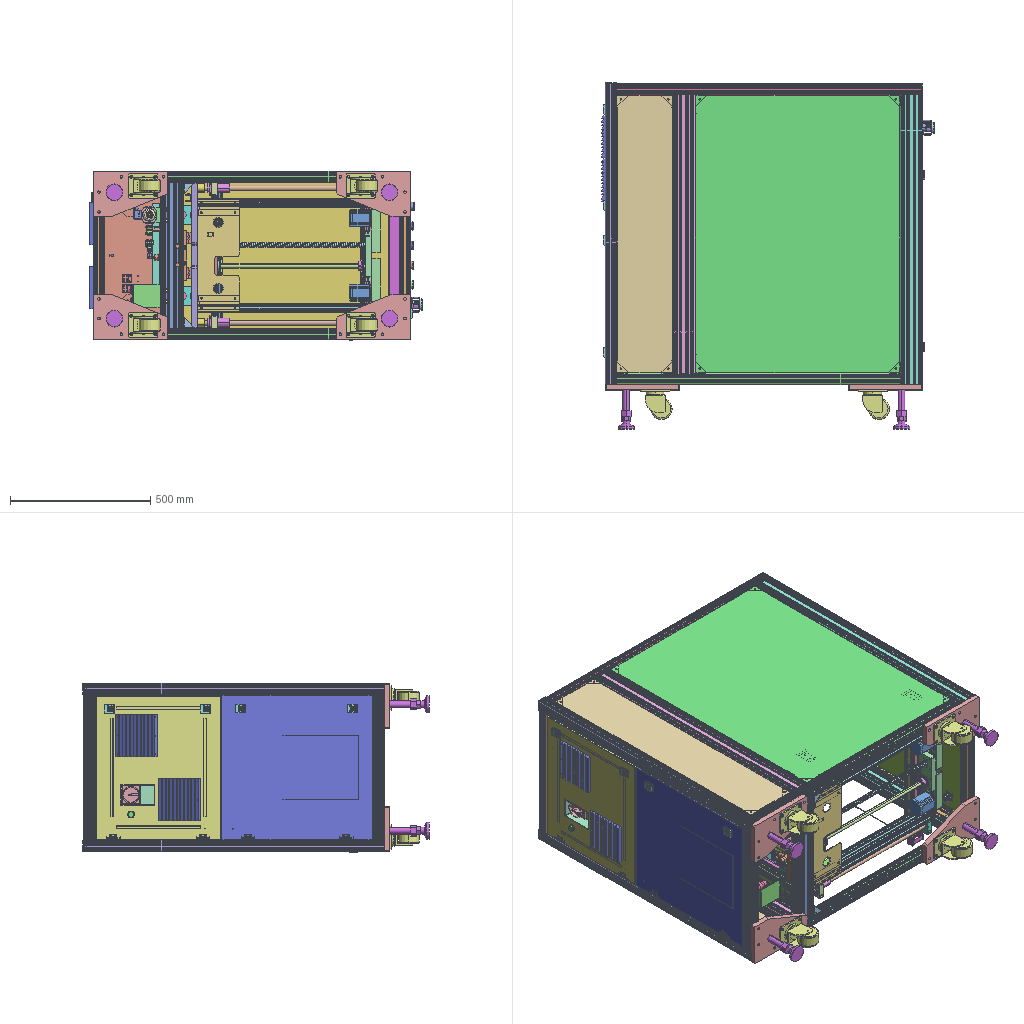Assembly | STEP file | 165 different items | 377 placed | box 1185 x 1234 x 604 mm
Parts list (item | name | quantity | parent item | size | volume):
1 | Caster support plate | x4 | - | 265 x 20 x 160 mm | 676074 mm3
2 | Fixing rod L520 | x2 | - | 520 x 40 x 80 mm | 414666 mm3
3 | Profile MK-8-4080H-L-05 4080H standard 990mm | x2 | - | 990 x 40 x 80 mm | 803657 mm3
4 | Profile MK-8-4080H-L-00 4080H standard 990mm | x2 | - | 990 x 40 x 80 mm | 803657 mm3
5 | - | x2 | - | 1030 x 40 x 80 mm | 836128 mm3
6 | Profile MK-8-4040C-L-00 4040C standard 520mm | x4 | - | 520 x 40 x 40 mm | 248689 mm3
7 | - | x2 | - | 1070 x 40 x 40 mm | 511726 mm3
8 | - | x2 | - | 1010 x 40 x 40 mm | 483031 mm3
9 | Profile MK-8-4040C-L-00 4040C standard 1086mm | x2 | - | 1086 x 40 x 40 mm | 519378 mm3
10 | - | x32 | - | 38 x 38 x 36 mm | 14409 mm3
11 | 3-inch heavy-duty caster 7223-222B | x4 | - | 112 x 105 x 88 mm | 158459 mm3
12 | - | x4 | - | 60 x 195 x 60 mm | 136685 mm3
13 | - | x2 | - | 40 x 12.4 x 40 mm | 4676 mm3
14 | - | x2 | - | 40 x 12.4 x 40 mm | 5038 mm3
15 | Door panel | x1 | - | 515 x 539 x 17 mm | 394918 mm3
16 | Hinge CL237Z3H001-01 | x6 | - | 17.5 x 48 x 18 mm | 5234 mm3
17 | - | x6 | - | 19 x 25 x 8.5 mm | 1495 mm3
18 | - | x1 | - | 230 x 270 x 19 mm | 66126 mm3
19 | - | x2 | in Lifting unit assembly | 199 x 989 x 30 mm | 288004 mm3
20 | - | x1 | in Lifting unit assembly | 199 x 519 x 30 mm | 154248 mm3
21 | Side seal plate large | x1 | in Lifting unit assembly | 988 x 728 x 30 mm | 958433 mm3
22 | - | x3 | in Lifting unit assembly | 71.855 x 71.5 x 21.7 mm | 42318 mm3
23 | Limit switch mounting plate | x2 | in Lifting unit assembly | 40 x 28 x 31 mm | 4364 mm3
24 | Cylinder fixing plate | x1 | in Lifting assembly | 95 x 15 x 180 mm | 203392 mm3
25 | Slider fixing plate | x1 | in Lifting assembly | 520 x 20 x 250 mm | 2234744 mm3
26 | Fixing block 1 | x2 | in Lifting assembly | 19 x 37 x 65 mm | 22556 mm3
27 | - | x1 | in Lifting assembly | 133 x 24 x 24 mm | 49135 mm3
28 | - | x1 | in Lifting assembly | 55 x 17 x 83 mm | 68793 mm3
29 | - | x2 | in Lifting assembly | 5.6 x 26 x 26 mm | 1190 mm3
30 | - | x2 | in Lifting assembly | 80 x 17 x 55 mm | 50244 mm3
31 | - | x2 | in Lifting assembly | 11.2 x 60 x 13 mm | 5055 mm3
32 | Fixing block 2 | x2 | in Lifting assembly | 40 x 35 x 35 mm | 25797 mm3
33 | - | x2 | in Lifting assembly | 68.92 x 68.92 x 20.5 mm | 34820 mm3
34 | - | x2 | in Lifting assembly | 12 x 42 x 42 mm | 7887 mm3
35 | - | x2 | in Support rail unit SBR30S2A+850L | 60 x 52 x 850 mm | 1179797 mm3
36 | - | x4 | in Support rail unit SBR30S2A+850L | 70 x 56 x 70 mm | 208407 mm3
37 | - | x5 | in Lifting assembly, Lifting unit assembly | 37.34 x 12.127 x 16.625 mm | 2631 mm3
38 | - | x4 | in Lifting assembly | 20 x 1 x 9 mm | 97.65 mm3
39 | - | x2 | in Lifting assembly | 16 x 16 x 8 mm | 1375 mm3
40 | - | x1 | in Lifting assembly | 494 x 75 x 75 mm | 957901 mm3
41 | Speed control valve with pilot-operated air lock ASP530F-03-08S | x1 | in Lifting assembly | 39.4 x 55.1 x 62.8 mm | 28936 mm3
42 | - | x1 | in Lifting assembly | 22.174 x 25.3 x 13.2 mm | 2514 mm3
43 | - | x1 | in Lifting assembly | 29.502 x 42.5 x 15.002 mm | 6910 mm3
44 | Speed control valve AS3201F-03-08SA | x1 | in Lifting assembly | 23 x 45.4 x 41 mm | 14301 mm3
45 | - | x2 | in Lifting assembly A_right | 620 x 30 x 60.001 mm | 358896 mm3
46 | Bottom adapter plate | x1 | in Lifting assembly A_right | 405 x 150 x 3 mm | 157925 mm3
47 | - | x2 | in Lifting assembly A_right | 60 x 12.2 x 30 mm | 5483 mm3
48 | Bearing fixing plate | x1 | - | 180 x 21 x 68 mm | 190682 mm3
49 | - | x1 | - | 170 x 21 x 57 mm | 135678 mm3
50 | - | x1 | - | 23 x 23 x 31.4 mm | 3535 mm3
51 | - | x1 | - | 16 x 647 x 16 mm | 120315 mm3
52 | - | x1 | - | 50.395 x 50.132 x 19 mm | 15455 mm3
53 | - | x1 | - | 50.395 x 50.132 x 19.5 mm | 13040 mm3
54 | - | x1 | - | 9 x 37 x 37 mm | 4601 mm3
55 | Shaft circlip type A 20 | x1 | - | 22.5 x 25.161 x 1 mm | 155.824 mm3
56 | Key 2 | x1 | - | 3.9 x 5.5 x 15 mm | 300.753 mm3
57 | - | x4 | - | 31 x 9 x 31 mm | 3611 mm3
58 | Deep groove ball bearing 606-ZZ | x8 | - | 6 x 17 x 17 mm | 776.566 mm3
59 | - | x8 | - | 18.3 x 17.603 x 1 mm | 85.781 mm3
60 | Chain sprocket spacer | x4 | - | 15 x 15 x 6.2 mm | 541.108 mm3
61 | - | x1 | - | 22 x 22 x 8 mm | 1773 mm3
62 | Bearing baffle | x2 | - | 40 x 30 x 2 mm | 1364 mm3
63 | Bearing 6000Z_P5_BONA_eco | x2 | - | 26 x 26 x 8 mm | 2544 mm3
64 | Bearing support plate | x1 | - | 12 x 35 x 135 mm | 43258 mm3
65 | -02 nut SFU01604-4 | x1 | - | 40 x 40 x 48 mm | 25660 mm3
66 | -01 screw pair SFUR1604-648 | x1 | - | 16 x 16 x 648 mm | 118967 mm3
67 | - | x1 | - | 13.6 x 15.973 x 1 mm | 68.14 mm3
68 | PN_0001 bearing 6001ZZ | x2 | - | 28 x 28 x 8 mm | 3776 mm3
69 | Motor fixing plate 2 | x2 | in Lifting assembly A_right | 68 x 152 x 35 mm | 46618 mm3
70 | - | x2 | in Lifting assembly A_right | 122.93 x 36.98 x 8 mm | 5373 mm3
71 | Stepper motor 24HS8404-10PJ3 | x2 | in Lifting assembly A_right | 60 x 96 x 60 mm | 237550 mm3
72 | Sliding plate 2 | x2 | in Lifting assembly A_right | 70 x 19 x 50 mm | 40709 mm3
73 | - | x2 | in Lifting assembly A_right | 80 x 54 x 38 mm | 45928 mm3
74 | Guide rod fixing plate 2 | x2 | in Lifting assembly A_right | 65 x 19 x 45 mm | 44231 mm3
75 | Guide shaft 2 | x2 | in Lifting assembly A_right | 20 x 20 x 616 mm | 193311 mm3
76 | - | x1 | in Lifting assembly A_right | 150 x 175 x 30 mm | 90977 mm3
77 | Right-angle fixing plate A | x1 | in Lifting assembly A_right | 150 x 175 x 30 mm | 91369 mm3
78 | - | x2 | in Lifting assembly A_right | 17.5 x 18 x 17.5 mm | 1873 mm3
79 | - | x2 | in Lifting assembly A_right | 37 x 19 x 37 mm | 15386 mm3
80 | - | x2 | in Lifting assembly A_right | 30 x 25 x 30 mm | 10205 mm3
81 | - | x1 | in Lifting assembly A_right | 22.7 x 14.9 x 13.4 mm | 1660 mm3
82 | - | x1 | in Lifting assembly A_right | 19.5 x 18 x 15 mm | 668.205 mm3
83 | - | x1 | in Lifting assembly A_right | 99 x 14.979 x 14.996 mm | 5984 mm3
84 | I/O distribution box 23N4S1 | x1 | in Lifting assembly A_right | 27.753 x 76.75 x 11.974 mm | 1445 mm3
85 | - | x4 | in Lifting assembly A_right | - | -
86 | - | x2 | in Lifting assembly A_right | 3 x 3 x 14 mm | 119.894 mm3
87 | Conveyor front chain guide groove L590 | x1 | in Conveyor assembly_right | 35 x 55 x 590 mm | 449690 mm3
88 | Conveyor rear chain guide groove L590 | x1 | in Conveyor assembly_right | 35 x 55 x 590 mm | 449690 mm3
89 | - | x2 | in Conveyor assembly_right | 9 x 490 x 20.4 mm | 77235 mm3
90 | - | x2 | in Conveyor assembly_right | 34.8 x 1 x 54.8 mm | 1804 mm3
91 | - | x2 | in Conveyor assembly_right | 34.8 x 1 x 54.8 mm | 1804 mm3
92 | - | x4 | - | 25 x 8.5 x 25 mm | 1521 mm3
93 | Driven guide wheel connector | x4 | in Conveyor assembly_right | 36 x 5 x 10.6 mm | 1667 mm3
94 | - | x4 | in Conveyor assembly_right | 15 x 15 x 3.5 mm | 281.21 mm3
95 | - | x2 | in Conveyor assembly_right | 18.325 x 9 x 17.4 mm | 854.513 mm3
96 | 06B side guide chain buckle | x2 | in Conveyor assembly_right | 15 x 1 x 7 mm | 49.292 mm3
97 | - | x2 | in Conveyor assembly_right, Lifting assembly A_right | 11.2 x 58.715 x 345.215 mm | 7993 mm3
98 | - | x2 | in Conveyor assembly_right | 20 x 10 x 20 mm | 2790 mm3
99 | Fixing plate 3 | x2 | in Conveyor assembly_right | 10 x 50 x 50 mm | 18064 mm3
100 | Photoelectric fixing plate 3 | x1 | in Conveyor assembly_right | 33 x 38 x 78 mm | 5566 mm3
101 | Photoelectric adapter plate 4 | x1 | in Lifting assembly A_right | 55 x 32 x 23.5 mm | 3494 mm3
102 | Adapter plate 3 | x4 | in Lifting unit assembly | 32 x 35 x 40 mm | 7142 mm3
103 | - | x2 | in Lifting unit assembly | 55 x 24.5 x 48.5 mm | 5670 mm3
104 | - | x1 | in Lifting unit assembly | 60 x 100 x 1.5 mm | 8744 mm3
105 | Polyurethane anti-collision column 2 | x4 | in Lifting unit assembly | 35 x 30 x 35 mm | 26422 mm3
106 | Cable carrier adapter plate 2 | x1 | in Lifting unit assembly | 35 x 35 x 37 mm | 4434 mm3
107 | - | x4 | in Lifting unit assembly | 30 x 30 x 1 mm | 412.566 mm3
108 | - | x4 | in Lifting unit assembly | 22 x 20 x 80 mm | 6135 mm3
109 | - | x2 | in Lifting unit assembly | 40 x 20 x 28 mm | 6776 mm3
110 | - | x1 | in Lifting unit assembly | 141.7 x 32.5 x 16 mm | 47379 mm3
111 | - | x1 | in Lifting unit assembly | 30 x 30 x 44.8 mm | 24470 mm3
112 | Pressure regulator filter GFR300-08-N | x1 | in Lifting unit assembly | - | -
113 | Hand slide valve HSV06 | x1 | in Lifting unit assembly | 27.5 x 27.5 x 50 mm | 15432 mm3
114 | Cylinder lock MS813-Shengjiu | x6 | in Lifting unit assembly | 58.793 x 35 x 31.6 mm | 16415 mm3
115 | Hydraulic buffer ACJ-1412 | x2 | in Lifting unit assembly | 19 x 100 x 21.289 mm | 13894 mm3
116 | - | x1 | - | 519 x 150 x 79 mm | 247371 mm3
117 | - | x1 | - | 40 x 40 x 48 mm | 24355 mm3
118 | - | x1 | - | 30 x 30 x 33 mm | 18043 mm3
119 | Pushbutton head LA42PD-Y | x2 | - | 30 x 30 x 76 mm | 18961 mm3
120 | Pushbutton head LA42PD-S | x1 | - | 30 x 30 x 33 mm | 18043 mm3
121 | - | x5 | - | 41 x 30 x 22 mm | 6377 mm3
122 | - | x5 | - | 32 x 10 x 42 mm | 10410 mm3
123 | Switch contact LA42-10-NO | x5 | - | 32 x 10 x 42 mm | 10410 mm3
124 | Emergency stop protective ring J-V | x1 | - | 47.915 x 30.4 x 47.915 mm | 9284 mm3
125 | Button cover plate | x1 | - | 519 x 39.5 x 206 mm | 125183 mm3
126 | Flashing buzzer AD17-SML-DC24V | x1 | - | 29 x 29 x 63 mm | 18875 mm3
127 | - | x1 | in Front sheet-metal door welded assembly | 515 x 796 x 17 mm | 556251 mm3
128 | - | x2 | in Front sheet-metal door welded assembly | 60 x 10 x 490 mm | 55944 mm3
129 | Electrical cabinet support plate | x1 | in Lifting unit assembly | 28 x 370 x 23 mm | 51078 mm3
130 | - | x2 | in Lifting unit assembly | 55 x 18 x 52 mm | 5293 mm3
131 | Limit fixing plate 2 | x1 | in Lifting unit assembly | 207 x 78 x 55 mm | 153668 mm3
132 | Connector fixing plate 2 | x1 | in Lifting unit assembly | 82 x 100 x 83 mm | 26763 mm3
133 | SMEMA connector | x2 | in Lifting unit assembly | 36 x 36 x 78.52 mm | 45655 mm3
134 | Face cover reinforcing rib 300mm | x2 | - | 300 x 21 x 6 mm | 7570 mm3
135 | - | x1 | - | 513 x 444 x 17 mm | 274646 mm3
136 | - | x2 | - | 350 x 21 x 6 mm | 8832 mm3
137 | Power knob mounting sheet metal | x1 | - | 74 x 122 x 41 mm | 24069 mm3
138 | - | x1 | - | 515 x 446 x 234 mm | 856637 mm3
139 | Class B ventilation filter mesh assembly ZL-803 (7032 glue) | x2 | - | 150 x 150 x 28 mm | 421271 mm3
140 | Control system fixing plate | x2 | - | 446 x 425 x 18 mm | 245891 mm3
141 | Power adapter plate 2 | x2 | - | 398 x 7.5 x 143 mm | 93935 mm3
142 | Power filter DL-10T1 | x1 | - | 89.5 x 36.5 x 51.5 mm | 121807 mm3
143 | Axial fan 1238A2MBL | x1 | - | 120 x 120 x 38 mm | 111801 mm3
144 | Six-position grounding copper block | x2 | - | 30.3 x 30.2 x 15 mm | 7115 mm3
145 | - | x1 | - | 24 x 37.7 x 24 mm | 7790 mm3
146 | - | x1 | - | 65.5 x 92 x 65.5 mm | 250369 mm3
147 | - | x1 | - | 54 x 38 x 11.5 mm | 8666 mm3
148 | Switching power supply LRS-50-24 (Mean Well) | x1 | - | 99 x 30 x 82 mm | 213867 mm3
149 | PLC module FX5U-32MT_ES | x1 | - | 150 x 96.4 x 84.9 mm | 980252 mm3
150 | Feed-through terminal block PT2,5-QUATTRO-3209578 | x20 | - | 5.15 x 72.2 x 35.25 mm | 9561 mm3
151 | Schneider miniature circuit breaker iDPNN-1P+N-C10A | x1 | - | 17.5 x 90.6 x 73.848 mm | 76092 mm3
152 | - | x1 | - | 35.4 x 93.9 x 74.3 mm | 159125 mm3
153 | Residual current device Vigi-iC65-ELE-2P-40A-30mA-A | x1 | - | 76.2 x 105.618 x 73.908 mm | 172404 mm3
154 | Switching power supply LRS-100-48 | x1 | - | 129 x 30 x 97 mm | 340596 mm3
155 | - | x2 | - | 119 x 77.6 x 25.5 mm | 99944 mm3
156 | - | x4 | - | 50.5 x 35.3 x 9.5 mm | 9735 mm3
157 | Rail socket EA9XN310 | x1 | - | 65.5 x 80.8 x 55 mm | 247844 mm3
158 | - | x3 | - | 80.625 x 35 x 371 mm | 72614 mm3
159 | 35 cable trunking (400) 2 | x2 | - | 80.625 x 35 x 425 mm | 83190 mm3
160 | - | x2 | - | 5.5 x 35 x 350 mm | 7332 mm3
161 | LED lighting lamp QELTS-300-220 220V 300mm | x1 | - | 37 x 33.2 x 378 mm | 378498 mm3
162 | - | x1 | in Acrylic cover plate assembly | 822 x 540 x 5 mm | 2219396 mm3
163 | Friction strip L824 | x2 | in Acrylic cover plate assembly | 7 x 11 x 824 mm | 22001 mm3
164 | Friction strip L542 | x2 | in Acrylic cover plate assembly | 7 x 11 x 542 mm | 14387 mm3
165 | Limit switch fixing plate 2 | x1 | in Lifting unit assembly | 40 x 26 x 30 mm | 4044 mm3
Placements (level | parent | child | x y z in mm | rotation matrix by rows), first 379 of 406 lines:
1 | Lifting unit assembly | subassembly 2 | 817.116 381.543 740.825 | 1 0 0 0 1 0 0 0 1
2 | subassembly 2 | Caster support plate | 950.319 429.73 717.441 | -1 0 0 0 1 0 0 0 -1
2 | subassembly 2 | Caster support plate | 950.319 429.73 1317.441 | -1 0 0 0 -1 0 0 0 1
2 | subassembly 2 | Caster support plate | -179.681 429.73 1317.441 | 1 0 0 0 1 0 0 0 1
2 | subassembly 2 | Caster support plate | -179.681 429.73 717.441 | 1 0 0 0 -1 0 0 0 -1
2 | subassembly 2 | Fixing rod L520 | 100.319 459.73 1277.441 | 0 0 1 0 1 0 -1 0 0
2 | subassembly 2 | Fixing rod L520 | 100.319 1489.73 757.441 | 0 0 1 0 -1 0 1 0 0
2 | subassembly 2 | Profile MK-8-4080H-L-05 4080H standard 990mm | 80.319 479.73 1161.941 | 0 -1 0 1 0 0 0 0 1
2 | subassembly 2 | Profile MK-8-4080H-L-05 4080H standard 990mm | 80.319 479.73 872.941 | 0 -1 0 1 0 0 0 0 1
2 | subassembly 2 | Profile MK-8-4080H-L-00 4080H standard 990mm | 100.319 479.73 737.441 | 0 0 1 1 0 0 0 1 -0
2 | subassembly 2 | Profile MK-8-4080H-L-00 4080H standard 990mm | 100.319 479.73 1297.441 | 0 0 1 1 0 0 0 1 -0
2 | subassembly 2 | subassembly 3 | 910.319 1469.73 1297.441 | 0 0 -1 -1 0 0 0 1 0
2 | subassembly 2 | subassembly 3 | 910.319 1469.73 737.441 | 0 0 -1 -1 0 0 0 1 0
2 | subassembly 2 | Profile MK-8-4040C-L-00 4040C standard 520mm | -159.681 459.73 757.441 | 0 0 -1 0 1 0 1 0 0
2 | subassembly 2 | Profile MK-8-4040C-L-00 4040C standard 520mm | 930.319 459.73 757.441 | 0 0 -1 0 1 0 1 0 0
2 | subassembly 2 | Profile MK-8-4040C-L-00 4040C standard 520mm | -159.681 1489.73 757.441 | 0 0 -1 0 1 0 1 0 0
2 | subassembly 2 | Profile MK-8-4040C-L-00 4040C standard 520mm | 930.319 1449.73 757.441 | 0 0 -1 0 1 0 1 0 0
2 | subassembly 2 | subassembly 4 | -159.681 439.73 1297.441 | 0 -1 0 1 0 0 0 0 1
2 | subassembly 2 | subassembly 5 | -139.681 459.73 1297.441 | 1 0 0 0 1 0 0 0 1
2 | subassembly 2 | subassembly 4 | -159.681 439.73 737.441 | 0 -1 0 1 0 0 0 0 1
2 | subassembly 2 | subassembly 5 | -139.681 459.73 737.441 | 1 0 0 0 1 0 0 0 1
2 | subassembly 2 | Profile MK-8-4040C-L-00 4040C standard 1086mm | -139.681 1489.73 1297.441 | 1 0 0 0 1 0 0 0 1
2 | subassembly 2 | Profile MK-8-4040C-L-00 4040C standard 1086mm | -139.681 1489.73 737.441 | 1 0 0 0 1 0 0 0 1
2 | subassembly 2 | subassembly 6 | -139.681 479.73 737.441 | 1 0 0 0 1 0 0 0 1
2 | subassembly 2 | subassembly 6 | -139.681 1469.73 737.441 | 0 1 0 -1 0 0 0 0 1
2 | subassembly 2 | subassembly 6 | 60.319 479.73 737.291 | 0 -1 0 1 0 0 0 0 1
2 | subassembly 2 | subassembly 6 | 60.319 1469.73 737.441 | -1 0 0 0 -1 0 0 0 1
2 | subassembly 2 | subassembly 6 | 140.319 479.73 737.291 | 1 0 0 0 1 0 0 0 1
2 | subassembly 2 | subassembly 6 | 140.319 1469.73 737.441 | 0 1 0 -1 0 0 0 0 1
2 | subassembly 2 | subassembly 6 | 870.319 479.73 737.441 | 0 -1 0 1 0 0 0 0 1
2 | subassembly 2 | subassembly 6 | 870.319 479.73 1297.291 | -1 0 0 0 1 0 0 0 -1
2 | subassembly 2 | subassembly 6 | 870.319 1469.73 1297.591 | 0 -1 0 -1 0 0 0 0 -1
2 | subassembly 2 | subassembly 6 | 140.319 1469.73 1297.441 | 1 0 0 0 -1 0 0 0 -1
2 | subassembly 2 | subassembly 6 | 140.319 479.73 1297.441 | 0 1 0 1 0 0 0 0 -1
2 | subassembly 2 | subassembly 6 | -139.681 1469.73 1297.441 | 1 0 0 0 -1 0 0 0 -1
2 | subassembly 2 | subassembly 6 | -139.681 479.73 1297.441 | 0 1 0 1 0 0 0 0 -1
2 | subassembly 2 | subassembly 6 | 60.319 479.73 1297.441 | -1 0 0 0 1 0 0 0 -1
2 | subassembly 2 | subassembly 6 | 60.319 1469.73 1297.441 | 0 -1 0 -1 0 0 0 0 -1
2 | subassembly 2 | subassembly 6 | 60.319 1489.73 1277.441 | -1 0 0 0 0 -1 0 -1 -0
2 | subassembly 2 | subassembly 6 | 60.319 1489.73 757.441 | 0 -1 0 0 0 -1 1 0 -0
2 | subassembly 2 | subassembly 6 | -139.681 1489.73 757.441 | 1 0 0 0 0 -1 0 1 0
2 | subassembly 2 | subassembly 6 | 60.319 459.73 1277.441 | -1 0 0 0 0 -1 0 -1 -0
2 | subassembly 2 | subassembly 6 | 60.319 459.73 757.441 | 0 -1 0 0 0 -1 1 0 0
2 | subassembly 2 | subassembly 6 | 140.319 459.73 1277.441 | 0 1 0 0 0 -1 -1 0 0
2 | subassembly 2 | 3-inch heavy-duty caster 7223-222B | 772.319 414.73 769.941 | -1 0 0 0 1 0 0 0 -1
2 | subassembly 2 | 3-inch heavy-duty caster 7223-222B | -1.681 414.73 769.941 | -1 0 0 0 1 0 0 0 -1
2 | subassembly 2 | 3-inch heavy-duty caster 7223-222B | 772.319 414.73 1264.941 | -1 0 0 0 1 0 0 0 -1
2 | subassembly 2 | 3-inch heavy-duty caster 7223-222B | -1.681 414.73 1264.941 | -1 0 0 0 1 0 0 0 -1
2 | subassembly 2 | subassembly 7 | 875.319 279.73 1242.441 | 1 0 0 0 1 0 0 0 1
2 | subassembly 2 | subassembly 7 | 875.319 279.73 792.441 | 1 0 0 0 1 0 0 0 1
2 | subassembly 2 | subassembly 7 | -104.681 279.73 792.441 | 1 0 0 0 1 0 0 0 1
2 | subassembly 2 | subassembly 7 | -104.681 279.73 1242.441 | 1 0 0.000641 0 1 0 -0.000641 0 1
2 | subassembly 2 | subassembly 6 | 80.169 1469.73 1277.441 | 0 0 -1 0 -1 0 -1 0 0
2 | subassembly 2 | subassembly 6 | 80.169 1469.73 757.441 | 0 0 -1 -1 0 0 0 1 -0
2 | subassembly 2 | subassembly 6 | -139.681 1489.73 1277.441 | 0 1 0 0 0 -1 -1 0 0
2 | subassembly 2 | subassembly 6 | 870.319 1469.73 737.441 | -1 0 0 0 -1 0 0 0 1
2 | subassembly 2 | subassembly 6 | 140.319 459.73 757.441 | 1 0 0 0 0 -1 0 1 0
2 | subassembly 2 | subassembly 6 | 910.319 1449.73 757.441 | -1 0 0 0 0 1 0 1 -0
2 | subassembly 2 | subassembly 6 | 910.319 1449.73 1277.441 | 0 -1 0 0 0 1 -1 0 -0
2 | subassembly 2 | subassembly 6 | 910.319 459.73 757.441 | 0 -1 0 0 0 -1 1 0 0
2 | subassembly 2 | subassembly 6 | 910.319 459.73 1277.441 | 0 -1 0 0 0 1 -1 0 -0
2 | subassembly 2 | subassembly 6 | -139.681 459.73 1277.441 | 0 1 0 0 0 -1 -1 0 0
2 | subassembly 2 | subassembly 6 | -139.681 459.73 757.441 | 1 0 0 0 0 -1 0 1 0
2 | subassembly 2 | subassembly 8 | 950.519 1489.73 1297.441 | 0 -1 0 -1 0 0 0 0 -1
2 | subassembly 2 | subassembly 8 | 950.519 1489.73 737.441 | 0 -1 0 1 0 0 0 0 1
2 | subassembly 2 | subassembly 9 | -159.681 1513.93 737.441 | -1 0 0 0 -1 0 0 0 1
2 | subassembly 2 | subassembly 9 | -159.681 1513.93 1297.441 | -1 0 0 0 -1 0 0 0 1
1 | Lifting unit assembly | subassembly 10 | 953.735 1175.238 2160.396 | 0 0 1 0 -1 0 1 0 -0
2 | subassembly 10 | Door panel | -402.579 43.466 -315.1 | -1 0 0 0 -1 0 0 0 1
2 | subassembly 10 | subassembly 11 | -628.948 -156.165 -270.668 | -1 0 0 0 1 0 0 0 -1
3 | subassembly 11 | Hinge CL237Z3H001-01 | 25.631 24.631 40.182 | 1 0 0 0 1 0 0 0 1
3 | subassembly 11 | subassembly 12 | 25.631 24.631 40.182 | -1 0 0 0 1 0 0 0 -1
2 | subassembly 10 | subassembly 11 | -628.948 193.835 -270.668 | -1 0 0 0 1 0 0 0 -1
3 | subassembly 11 | Hinge CL237Z3H001-01 | 25.631 24.631 40.182 | 1 0 0 0 1 0 0 0 1
3 | subassembly 11 | subassembly 12 | 25.631 24.631 40.182 | -1 0 0 0 1 0 0 0 -1
2 | subassembly 10 | subassembly 13 | -402.579 127.966 -296.1 | -1 0 0 0 -1 0 0 0 1
1 | Lifting unit assembly | subassembly 14 | 777.434 1356.272 1459.067 | -1 0 0 0 1 0 0 0 -1
1 | Lifting unit assembly | subassembly 14 | 777.434 1356.272 2057.466 | 1 0 0 0 1 0 0 0 1
1 | Lifting unit assembly | subassembly 15 | 777.434 1890.472 1758.266 | 1 0 0 0 0 1 0 -1 0
1 | Lifting unit assembly | Side seal plate large | 1322.434 1356.272 2058.266 | 0 1 0 -1 0 0 0 0 1
1 | Lifting unit assembly | subassembly 16 | 1060.134 1830.272 1511.617 | -1 0 0 0 1 0 0 0 -1
1 | Lifting unit assembly | Limit switch mounting plate | 1047.434 1837.272 1498.767 | -1 0 0 0 1 0 0 0 -1
1 | Lifting unit assembly | Lifting assembly A_right | 994.3 1296.677 1735.039 | 1 0 0 0 1 0 0 0 1
2 | Lifting assembly A_right | Lifting assembly | -1579.962 -1409.405 569.136 | 1 0 0 0 1 0 0 0 1
3 | Lifting assembly | Cylinder fixing plate | 1508.097 974.0 -545.909 | -1 0 0 0 1 0 0 0 -1
3 | Lifting assembly | Slider fixing plate | 1573.097 1124.0 -545.909 | 0 1 0 0 0 -1 -1 0 0
3 | Lifting assembly | Fixing block 1 | 1510.597 999.0 -608.409 | 0 0 1 0 1 0 -1 0 -0
3 | Lifting assembly | Fixing block 1 | 1510.597 999.0 -483.409 | 0 0 1 0 1 0 -1 0 -0
3 | Lifting assembly | subassembly 17 | 1518.097 1526.0 -545.909 | 0 -0.2484 -0.9687 0 -0.9687 0.2484 -1 0 -0
3 | Lifting assembly | subassembly 18 | 1518.097 1476.0 -545.909 | 1 0 0 0 -1 0 0 0 -1
3 | Lifting assembly | subassembly 19 | 1518.097 1526.0 -500.309 | 0 0.3457 0.9383 0 0.9383 -0.3457 -1 0 0
3 | Lifting assembly | subassembly 19 | 1518.097 1526.0 -585.909 | 0 0.8733 0.4872 0 0.4872 -0.8733 -1 0 0
3 | Lifting assembly | subassembly 20 | 1518.097 1516.0 -578.909 | 0 0 1 -1 0 0 0 -1 0
3 | Lifting assembly | subassembly 20 | 1518.097 1516.0 -512.909 | 0 0 -1 -1 0 0 0 1 -0
3 | Lifting assembly | subassembly 21 | 1551.097 1066.5 -483.409 | 0 0 1 0 1 0 -1 0 -0
3 | Lifting assembly | subassembly 21 | 1551.097 1066.5 -608.409 | 0 0 1 0 1 0 -1 0 -0
3 | Lifting assembly | Fixing block 2 | 1555.597 1059.0 -483.409 | 0 0 1 0 -1 0 1 0 0
3 | Lifting assembly | Fixing block 2 | 1555.597 1059.0 -608.409 | 0 0 1 0 -1 0 1 0 -0
3 | Lifting assembly | subassembly 22 | 1518.097 1526.0 -608.409 | 0.601 0.7992 0 0.7992 -0.601 0 0 0 -1
3 | Lifting assembly | subassembly 23 | 1518.097 1526.0 -511.909 | 0 -0.235 -0.972 0 -0.972 0.235 -1 0 -0
3 | Lifting assembly | subassembly 23 | 1518.097 1526.0 -579.909 | 0 -0.235 -0.972 0 -0.972 0.235 -1 0 -0
3 | Lifting assembly | subassembly 22 | 1518.097 1526.0 -483.409 | -0.601 0.7992 0 -0.7992 -0.601 0 0 0 1
3 | Lifting assembly | Support rail unit SBR30S2A+850L | 1540.097 1434.0 -401.409 | 0 1 0 0 0 -1 -1 0 -0
4 | Support rail unit SBR30S2A+850L | subassembly 24 | -0.0 -0.0 -0.0 | 1 0 0 0 1 0 0 0 1
4 | Support rail unit SBR30S2A+850L | subassembly 25 | 0.0 -0.0 220.0 | 1 0 0 0 1 0 0 0 1
4 | Support rail unit SBR30S2A+850L | subassembly 25 | 0.0 -0.0 385.0 | 1 0 0 0 1 0 0 0 1
3 | Lifting assembly | Support rail unit SBR30S2A+850L | 1540.097 1434.0 -690.409 | 0 1 0 0 0 -1 -1 0 -0
4 | Support rail unit SBR30S2A+850L | subassembly 24 | -0.0 -0.0 -0.0 | 1 0 0 0 1 0 0 0 1
4 | Support rail unit SBR30S2A+850L | subassembly 25 | 0.0 -0.0 220.0 | 1 0 0 0 1 0 0 0 1
4 | Support rail unit SBR30S2A+850L | subassembly 25 | 0.0 -0.0 385.0 | 1 0 0 0 1 0 0 0 1
3 | Lifting assembly | subassembly 26 | 1496.243 1009.121 -608.409 | 0 1 0 -1 0 0 0 0 1
3 | Lifting assembly | subassembly 27 | 1485.125 1026.85 -616.834 | -0.004456 0 -1 -1 0 0.004456 0 1 0
3 | Lifting assembly | subassembly 26 | 1496.243 1009.121 -483.409 | 0 1 0 -1 0 0 0 0 1
3 | Lifting assembly | subassembly 27 | 1485.125 1026.85 -491.834 | -0.004456 0 -1 -1 0 0.004456 0 1 0
3 | Lifting assembly | subassembly 28 | 1551.097 1053.5 -483.409 | 0.6856 0.728 0 0 0 1 0.728 -0.6856 -0
3 | Lifting assembly | subassembly 28 | 1551.097 1053.5 -608.409 | 0.6856 0.728 0 0 0 1 0.728 -0.6856 -0
3 | Lifting assembly | subassembly 27 | 1551.069 1096.85 -599.984 | 0.004456 0 1 -1 0 0.004456 0 -1 -0
3 | Lifting assembly | subassembly 26 | 1539.951 1079.121 -608.409 | 0 -1 0 -1 0 0 0 0 -1
3 | Lifting assembly | subassembly 27 | 1551.069 1096.85 -474.984 | 0.004456 0 1 -1 0 0.004456 0 -1 -0
3 | Lifting assembly | subassembly 26 | 1539.951 1079.121 -483.409 | 0 -1 0 -1 0 0 0 0 -1
3 | Lifting assembly | subassembly 29 | 1518.097 1410.0 -545.909 | 0 0 -1 -1 0 0 0 1 0
3 | Lifting assembly | Speed control valve with pilot-operated air lock ASP530F-03-08S | 1485.497 1005.5 -553.409 | 0 -1 0 0 0 -1 1 0 -0
3 | Lifting assembly | subassembly 30 | 1438.247 1005.5 -553.409 | 0 -1 0 0.5 0 -0.866 0.866 0 0.5
3 | Lifting assembly | subassembly 31 | 1422.647 1031.45 -508.462 | 1 0 0 0 0.5 -0.866 0 0.866 0.5
3 | Lifting assembly | Speed control valve AS3201F-03-08SA | 1485.297 1393.5 -553.409 | 0 -1 0 0.943 0 -0.3328 0.3328 0 0.943
2 | Lifting assembly A_right | subassembly 32 | 13.135 -380.405 210.728 | 1 0 0 0 0 -1 0 1 -0
2 | Lifting assembly A_right | subassembly 32 | 13.135 -380.405 -164.272 | 1 0 0 0 0 -1 0 1 -0
2 | Lifting assembly A_right | Bottom adapter plate | 88.135 -410.405 23.228 | 0 -1 0 0 0 1 -1 0 0
2 | Lifting assembly A_right | subassembly 33 | 637.135 -380.405 210.728 | 0 -1 0 1 0 0 0 0 1
2 | Lifting assembly A_right | subassembly 33 | 637.135 -380.405 -164.272 | 0 -1 0 1 0 0 0 0 1
2 | Lifting assembly A_right | subassembly 34 | 203.126 -373.279 -397.598 | 0 -1 0 0 0 1 -1 0 0
3 | subassembly 34 | Bearing fixing plate | -418.325 -418.509 -11.126 | 1 0 0 0 1 0 0 0 1
3 | subassembly 34 | subassembly 35 | -413.325 128.491 -5.626 | 1 0 0 0 1 0 0 0 1
3 | subassembly 34 | subassembly 36 | -383.325 106.991 -12.126 | 0.8521 0.5234 0 0 0 1 0.5234 -0.8521 -0
3 | subassembly 34 | subassembly 37 | -383.325 -136.509 -12.126 | 0.5234 0 -0.8521 0 -1 0 -0.8521 0 -0.5234
3 | subassembly 34 | subassembly 38 | -383.325 -399.509 -12.126 | 0.03301 0.9995 0 0 0 -1 -0.9995 0.03301 -0
3 | subassembly 34 | subassembly 39 | -383.325 109.491 -12.126 | -0.09776 -0.9952 0 0 0 -1 0.9952 -0.09776 0
3 | subassembly 34 | subassembly 40 | -383.325 130.991 -12.126 | 0 -0.1125 0.9936 -1 0 0 0 -0.9936 -0.1125
3 | subassembly 34 | Shaft circlip type A 20 | -382.696 135.991 -11.897 | -0.342 0.9397 0 0 0 1 0.9397 0.342 -0
3 | subassembly 34 | Key 2 | -387.905 108.941 -4.67 | -0.8521 -0.5234 0 0 0 1 -0.5234 0.8521 -0
3 | subassembly 34 | subassembly 41 | -313.591 -372.036 27.854 | 0.4469 0 -0.8946 0 -1 0 -0.8946 0 -0.4469
4 | subassembly 41 | subassembly 42 | -6.597 27.473 34.415 | 1 0 0 0 1 0 0 0 1
4 | subassembly 41 | Deep groove ball bearing 606-ZZ | -6.597 26.773 34.415 | 0 1 0 -1 0 0 0 0 1
4 | subassembly 41 | subassembly 43 | -6.597 30.473 34.415 | 1 0 0 0 0 -1 0 1 -0
3 | subassembly 34 | Chain sprocket spacer | -347.325 -408.009 18.374 | -0.09332 0.9956 0 0 0 1 0.9956 0.09332 -0
3 | subassembly 34 | Chain sprocket spacer | -419.325 -408.009 18.374 | -0.09332 0.9956 0 0 0 1 0.9956 0.09332 -0
3 | subassembly 34 | subassembly 41 | -385.591 -372.036 27.854 | 0.4469 0 -0.8946 0 -1 0 -0.8946 0 -0.4469
4 | subassembly 41 | subassembly 42 | -6.597 27.473 34.415 | 1 0 0 0 1 0 0 0 1
4 | subassembly 41 | Deep groove ball bearing 606-ZZ | -6.597 26.773 34.415 | 0 1 0 -1 0 0 0 0 1
4 | subassembly 41 | subassembly 43 | -6.597 30.473 34.415 | 1 0 0 0 0 -1 0 1 -0
3 | subassembly 34 | Chain sprocket spacer | -419.325 117.991 18.374 | -0.354 -0.9352 0 0 0 -1 0.9352 -0.354 0
3 | subassembly 34 | Chain sprocket spacer | -347.325 117.991 18.374 | -0.354 -0.9352 0 0 0 -1 0.9352 -0.354 0
3 | subassembly 34 | subassembly 41 | -448.621 82.019 -0.8524 | 0.3815 0 0.9244 0 1 0 -0.9244 0 0.3815
4 | subassembly 41 | subassembly 42 | -6.597 27.473 34.415 | 1 0 0 0 1 0 0 0 1
4 | subassembly 41 | Deep groove ball bearing 606-ZZ | -6.597 26.773 34.415 | 0 1 0 -1 0 0 0 0 1
4 | subassembly 41 | subassembly 43 | -6.597 30.473 34.415 | 1 0 0 0 0 -1 0 1 -0
3 | subassembly 34 | subassembly 41 | -370.973 82.019 -7.485 | 0.5977 0 0.8017 0 1 0 -0.8017 0 0.5977
4 | subassembly 41 | subassembly 42 | -6.597 27.473 34.415 | 1 0 0 0 1 0 0 0 1
4 | subassembly 41 | Deep groove ball bearing 606-ZZ | -6.597 26.773 34.415 | 0 1 0 -1 0 0 0 0 1
4 | subassembly 41 | subassembly 43 | -6.597 30.473 34.415 | 1 0 0 0 0 -1 0 1 -0
3 | subassembly 34 | subassembly 42 | -458.325 -437.009 -12.126 | -0.3217 0.9468 0 0 0 1 0.9468 0.3217 -0
3 | subassembly 34 | Bearing baffle | -458.325 -429.009 -12.126 | 1 0 0 0 0 1 0 -1 -0
3 | subassembly 34 | Bearing 6000Z_P5_BONA_eco | -458.325 185.991 -12.126 | -0.9239 -0.3826 0 0 0 -1 0.3826 -0.9239 -0
3 | subassembly 34 | Bearing support plate | -420.825 177.991 -12.126 | 0 0 -1 1 0 0 0 -1 0
3 | subassembly 34 | Bearing 6000Z_P5_BONA_eco | -383.325 185.991 -12.126 | 0.8583 0.5132 0 0 0 -1 -0.5132 0.8583 0
3 | subassembly 34 | subassembly 44 | -481.56 -333.951 -7.12 | -0.9237 -0.383 0 0 0 -1 0.383 -0.9237 0
4 | subassembly 44 | -02 nut SFU01604-4 | -23.38 -4.276 -481.942 | 0 -0.383 0.9237 0 0.9237 0.383 -1 0 -0
4 | subassembly 44 | -01 screw pair SFUR1604-648 | -23.38 -4.276 87.058 | -0.9237 -0.383 0 -0.383 0.9237 0 0 0 -1
3 | subassembly 34 | Bearing baffle | -383.325 -429.009 -12.126 | 1 0 0 0 0 1 0 -1 -0
3 | subassembly 34 | subassembly 45 | -383.748 -429.509 -12.046 | -0.1847 -0.9828 0 0 0 1 -0.9828 0.1847 -0
3 | subassembly 34 | PN_0001 bearing 6001ZZ | -383.325 -416.509 -12.126 | -0.6507 0.7593 0 0 0 1 0.7593 0.6507 -0
3 | subassembly 34 | PN_0001 bearing 6001ZZ | -458.325 -416.509 -12.126 | -0.6507 0.7593 0 0 0 1 0.7593 0.6507 -0
2 | Lifting assembly A_right | Motor fixing plate 2 | 667.135 -385.405 110.228 | 0 0 -1 1 0 0 0 -1 0
2 | Lifting assembly A_right | subassembly 46 | 641.635 -385.405 -14.272 | 0 0 1 0 1 0 -1 0 -0
2 | Lifting assembly A_right | Stepper motor 24HS8404-10PJ3 | 557.135 -385.405 -109.772 | 0 1 0 0 0 -1 -1 0 -0
2 | Lifting assembly A_right | subassembly 46 | 641.635 -385.405 60.728 | 0 0 1 0 -1 0 1 0 -0
2 | Lifting assembly A_right | Stepper motor 24HS8404-10PJ3 | 557.135 -385.405 156.228 | 0 1 0 0 0 -1 -1 0 -0
2 | Lifting assembly A_right | Sliding plate 2 | 74.635 -375.405 263.228 | 0 1 0 0 0 1 1 0 0
2 | Lifting assembly A_right | subassembly 47 | 49.135 -375.405 263.228 | 1 0 0 0 0 -1 0 1 -0
2 | Lifting assembly A_right | Guide rod fixing plate 2 | 621.635 -372.905 263.228 | 0 -1 0 0 0 1 -1 0 0
2 | Lifting assembly A_right | Guide shaft 2 | 620.135 -375.405 263.228 | 0 0 -1 -0.4984 -0.8669 0 -0.8669 0.4984 0
2 | Lifting assembly A_right | Guide rod fixing plate 2 | 621.635 -372.905 -216.772 | 0 -1 0 0 0 1 -1 0 0
2 | Lifting assembly A_right | Guide shaft 2 | 620.135 -375.405 -216.772 | 0 0 -1 -0.6082 0.7938 0 0.7938 0.6082 0
2 | Lifting assembly A_right | subassembly 47 | 49.135 -375.405 -216.772 | 1 0 0 0 0 1 0 -1 0
2 | Lifting assembly A_right | Sliding plate 2 | 74.635 -375.405 -216.772 | 0 1 0 0 0 1 1 0 0
2 | Lifting assembly A_right | subassembly 48 | 43.135 -352.405 190.728 | -1 0 0 0 1 0 0 0 -1
2 | Lifting assembly A_right | Right-angle fixing plate A | 43.135 -352.405 -149.272 | -1 0 0 0 1 0 0 0 -1
2 | Lifting assembly A_right | subassembly 49 | 638.635 -385.405 156.228 | 0 1 0 -0.3663 0 -0.9305 -0.9305 0 0.3663
2 | Lifting assembly A_right | subassembly 50 | 650.635 -385.405 60.728 | 0 1 0 0 0 1 1 0 0
2 | Lifting assembly A_right | Motor fixing plate 2 | 667.135 -385.405 -63.772 | 0 0 -1 -1 0 0 0 1 0
2 | Lifting assembly A_right | subassembly 51 | 38.135 -375.405 263.228 | 0 -1 0 0.8179 0 0.5754 -0.5754 0 0.8179
2 | Lifting assembly A_right | subassembly 52 | 61.135 -397.505 95.228 | 1 0 0 0 1 0 0 0 1
2 | Lifting assembly A_right | subassembly 53 | 65.635 -393.405 85.228 | 0 1 0 1 0 0 0 0 -1
2 | Lifting assembly A_right | subassembly 51 | 38.135 -375.405 -216.772 | 0 -1 0 0.32 0 0.9474 -0.9474 0 0.32
2 | Lifting assembly A_right | subassembly 54 | 62.735 -372.416 139.159 | 0 0.7572 0.6531 0 -0.6531 0.7572 1 0 0
2 | Lifting assembly A_right | I/O distribution box 23N4S1 | 128.585 -372.406 189.878 | 0.000147 -1 0 -1 -0.000147 0 0 0 -1
2 | Lifting assembly A_right | subassembly 55 | 104.636 -380.659 162.878 | 0.3271 0 -0.945 0.945 0 0.3271 0 -1 0
2 | Lifting assembly A_right | subassembly 55 | 126.636 -380.656 162.878 | -0.6482 0 0.7615 -0.7615 0 -0.6482 0 -1 -0
2 | Lifting assembly A_right | subassembly 55 | 115.634 -364.158 162.878 | -0.6482 0 0.7615 -0.7615 0 -0.6482 0 -1 -0
2 | Lifting assembly A_right | subassembly 55 | 93.634 -364.161 162.878 | 0.2554 0 -0.9668 0.9668 0 0.2554 0 -1 0
2 | Lifting assembly A_right | subassembly 50 | 650.635 -385.405 -14.272 | 0 1 0 0.5234 0 -0.8521 -0.8521 0 -0.5234
2 | Lifting assembly A_right | subassembly 56 | 653.635 -381.4 -11.813 | 0 0 1 0.5234 0.8521 0 -0.8521 0.5234 -0
2 | Lifting assembly A_right | subassembly 56 | 653.135 -390.105 60.728 | 0 0 1 0 1 0 -1 0 -0
2 | Lifting assembly A_right | subassembly 49 | 635.135 -385.405 -109.772 | 0 1 0 -0.937 0 0.3494 0.3494 0 0.937
2 | Lifting assembly A_right | Conveyor assembly_right | 601.135 -319.82 23.228 | 0 0 1 0 1 0 -1 0 -0
3 | Conveyor assembly_right | Conveyor front chain guide groove L590 | -0.0 -0.0 0.0 | 0 0 1 0 1 0 -1 0 -0
3 | Conveyor assembly_right | Conveyor rear chain guide groove L590 | -0.0 0.0 -506.0 | 0 0 -1 0 1 0 1 0 -0
3 | Conveyor assembly_right | subassembly 57 | -0.0 1.115 -3.5 | 0 -1 0 0 0 -1 1 0 0
3 | Conveyor assembly_right | subassembly 57 | -0.0 1.115 -502.5 | 0 1 0 0 0 -1 -1 0 0
3 | Conveyor assembly_right | subassembly 58 | -296.0 -3.085 -520.5 | 0 1 0 0 0 -1 -1 0 0
3 | Conveyor assembly_right | subassembly 58 | 296.0 -3.085 14.5 | 0 -1 0 0 0 -1 1 0 -0
3 | Conveyor assembly_right | subassembly 59 | -296.0 -3.085 14.5 | 0 1 0 0 0 1 1 0 0
3 | Conveyor assembly_right | subassembly 59 | 296.0 -3.085 -520.5 | 0 -1 0 0 0 1 -1 0 -0
3 | Conveyor assembly_right | subassembly 60 | 245.813 21.773 -24.973 | 0.4736 0 0.8808 0.8808 0 -0.4736 0 1 -0
4 | subassembly 60 | subassembly 42 | -6.597 27.473 34.415 | 1 0 0 0 1 0 0 0 1
4 | subassembly 60 | Deep groove ball bearing 606-ZZ | -6.597 26.473 34.415 | 0 1 0 -1 0 0 0 0 1
4 | subassembly 60 | subassembly 43 | -6.597 30.023 34.415 | 1 0 0 0 0 -1 0 1 0
3 | Conveyor assembly_right | subassembly 60 | -261.546 34.279 -481.027 | -0.9409 0 -0.3388 0.3388 0 -0.9409 0 -1 -0
4 | subassembly 60 | subassembly 42 | -6.597 27.473 34.415 | 1 0 0 0 1 0 0 0 1
4 | subassembly 60 | Deep groove ball bearing 606-ZZ | -6.597 26.473 34.415 | 0 1 0 -1 0 0 0 0 1
4 | subassembly 60 | subassembly 43 | -6.597 30.023 34.415 | 1 0 0 0 0 -1 0 1 0
3 | Conveyor assembly_right | subassembly 60 | 234.699 13.249 -481.027 | -0.5543 0 0.8323 -0.8323 0 -0.5543 0 -1 0
4 | subassembly 60 | subassembly 42 | -6.597 27.473 34.415 | 1 0 0 0 1 0 0 0 1
4 | subassembly 60 | Deep groove ball bearing 606-ZZ | -6.597 26.473 34.415 | 0 1 0 -1 0 0 0 0 1
4 | subassembly 60 | subassembly 43 | -6.597 30.023 34.415 | 1 0 0 0 0 -1 0 1 0
3 | Conveyor assembly_right | subassembly 60 | -243.44 18.483 -24.973 | 0.6862 0 -0.7274 -0.7274 0 -0.6862 0 1 0
4 | subassembly 60 | subassembly 42 | -6.597 27.473 34.415 | 1 0 0 0 1 0 0 0 1
4 | subassembly 60 | Deep groove ball bearing 606-ZZ | -6.597 26.473 34.415 | 0 1 0 -1 0 0 0 0 1
4 | subassembly 60 | subassembly 43 | -6.597 30.023 34.415 | 1 0 0 0 0 -1 0 1 0
3 | Conveyor assembly_right | Driven guide wheel connector | -261.0 -0.335 15.5 | -1 0 0 0 0 1 0 1 0
3 | Conveyor assembly_right | Driven guide wheel connector | -255.0 -0.335 -516.5 | -1 0 0 0 0 1 0 1 -0
3 | Conveyor assembly_right | Driven guide wheel connector | 261.0 -0.335 15.5 | 1 0 0 0 0 -1 0 1 0
3 | Conveyor assembly_right | Driven guide wheel connector | 255.0 -0.335 -516.5 | 1 0 0 0 0 -1 0 1 0
3 | Conveyor assembly_right | subassembly 61 | -273.0 -0.335 8.0 | -0.2046 -0.9788 0 -0.9788 0.2046 0 0 0 -1
3 | Conveyor assembly_right | subassembly 61 | -267.0 -0.335 -514.0 | 0.564 -0.8258 0 0.8258 0.564 0 0 0 1
3 | Conveyor assembly_right | subassembly 61 | 267.0 -0.335 -514.0 | 0.564 -0.8258 0 0.8258 0.564 0 0 0 1
3 | Conveyor assembly_right | subassembly 61 | 273.0 -0.335 8.0 | -0.2046 -0.9788 0 -0.9788 0.2046 0 0 0 -1
3 | Conveyor assembly_right | subassembly 62 | 47.065 15.415 -7.44 | -1 0 0 0 1 0 0 0 -1
3 | Conveyor assembly_right | 06B side guide chain buckle | 49.751 19.348 -3.44 | 0.564 0 0.8258 0.8258 0 -0.564 0 1 0
3 | Conveyor assembly_right | 06B side guide chain buckle | -54.952 11.331 -503.56 | 0.1764 0 0.9843 0.9843 0 -0.1764 0 1 -0
3 | Conveyor assembly_right | subassembly 62 | -51.343 15.065 -498.56 | 0.467 -0.8842 0 0.8842 0.467 0 0 0 1
3 | Conveyor assembly_right | subassembly 63 | 279.5 -35.585 -38.9 | 0 1 0 0 0 1 1 0 0
3 | Conveyor assembly_right | subassembly 64 | -281.0 29.415 -494.1 | 0 1 0 0.766 0 -0.6428 -0.6428 0 -0.766
3 | Conveyor assembly_right | subassembly 64 | -281.0 29.415 -11.9 | 0 1 0 -0.9385 0 0.3454 0.3454 0 0.9385
3 | Conveyor assembly_right | Fixing plate 3 | -271.0 34.415 6.6 | 0 1 0 -1 0 0 0 0 1
3 | Conveyor assembly_right | Fixing plate 3 | -271.0 24.415 -512.6 | 0 1 0 1 0 0 0 0 -1
3 | Conveyor assembly_right | Photoelectric fixing plate 3 | 286.0 -58.585 -20.5 | -1 0 0 0 1 0 0 0 -1
2 | Lifting assembly A_right | Photoelectric adapter plate 4 | 572.135 -380.405 249.228 | 0 -1 0 -1 0 0 0 0 -1
2 | Lifting assembly A_right | subassembly 63 | 549.635 -351.405 242.128 | 0 1 0 0 0 1 1 0 0
1 | Lifting unit assembly | Adapter plate 3 | 677.434 1776.272 2015.766 | 0 1 0 0 0 1 1 0 -0
1 | Lifting unit assembly | Adapter plate 3 | 677.434 1776.272 1500.766 | 0 1 0 0 0 -1 -1 0 0
1 | Lifting unit assembly | subassembly 65 | 666.684 1331.322 2016.766 | 0 1 0 1 0 0 0 0 -1
1 | Lifting unit assembly | subassembly 65 | 666.684 903.022 2016.766 | 0 1 0 1 0 0 0 0 -1
1 | Lifting unit assembly | subassembly 66 | 877.434 1217.281 1861.266 | -1 0 0 0 1 0 0 0 -1
1 | Lifting unit assembly | Polyurethane anti-collision column 2 | 917.434 878.772 1922.766 | 0 1 0 -0.9599 0 -0.2802 -0.2802 0 0.9599
1 | Lifting unit assembly | Polyurethane anti-collision column 2 | 917.434 878.772 1593.766 | 0 1 0 0.00389 0 -1 -1 0 -0.00389
1 | Lifting unit assembly | Cable carrier adapter plate 2 | 907.671 1263.772 1960.266 | 0 0 -1 1 0 0 0 -1 0
1 | Lifting unit assembly | subassembly 67 | 638.635 933.272 1967.317 | 0 0 1 0 -1 0 1 0 -0
1 | Lifting unit assembly | subassembly 67 | 638.635 1330.272 1967.317 | 0 0 1 0 -1 0 1 0 -0
1 | Lifting unit assembly | subassembly 68 | 664.135 1306.772 1501.267 | 1 0 0 0 0 -1 0 1 -0
1 | Lifting unit assembly | subassembly 68 | 664.135 956.772 1501.267 | 1 0 0 0 0 -1 0 1 -0
1 | Lifting unit assembly | subassembly 69 | 909.671 1233.272 1976.266 | 0 1 0 1 0 0 0 0 -1
1 | Lifting unit assembly | subassembly 69 | 987.434 950.772 1950.266 | 0 -1 0 1 0 0 0 0 1
1 | Lifting unit assembly | subassembly 70 | 859.434 1217.281 1853.266 | 0 -1 0 -1 0 0 0 0 -1
1 | Lifting unit assembly | subassembly 71 | 783.434 1078.272 1902.766 | 0 0 -1 0 1 0 1 0 -0
1 | Lifting unit assembly | Pressure regulator filter GFR300-08-N | 836.434 1078.272 1902.766 | -1 0 0 0 1 0 0 0 -1
1 | Lifting unit assembly | Hand slide valve HSV06 | 836.434 1078.272 1833.366 | 0.8827 -0.4699 0 0.4699 0.8827 0 0 0 1
1 | Lifting unit assembly | Cylinder lock MS813-Shengjiu | 637.434 1331.322 1967.817 | 0 0 -1 0 1 0 1 0 0
1 | Lifting unit assembly | Cylinder lock MS813-Shengjiu | 637.434 933.272 1967.817 | 0 0 -1 0 1 0 1 0 0
1 | Lifting unit assembly | Hydraulic buffer ACJ-1412 | 940.434 1540.234 1725.766 | -0.4711 0 0.8821 0 -1 0 0.8821 0 0.4711
1 | Lifting unit assembly | Hydraulic buffer ACJ-1412 | 940.434 1540.234 1790.766 | 0.692 0 0.7219 0 -1 0 0.7219 0 -0.692
1 | Lifting unit assembly | subassembly 72 | 1397.508 1465.42 2035.612 | 0 0 1 0 1 0 -1 0 -0
2 | subassembly 72 | subassembly 73 | 277.346 269.852 369.926 | 1 0 0 0 1 0 0 0 1
2 | subassembly 72 | subassembly 74 | 452.346 269.852 411.926 | -0.7991 0.6012 0 0.6012 0.7991 0 0 0 -1
2 | subassembly 72 | subassembly 75 | 312.346 269.852 378.926 | -0.1349 0.9909 0 0.9909 0.1349 0 0 0 -1
2 | subassembly 72 | Pushbutton head LA42PD-Y | 242.346 269.852 378.926 | 0.4933 -0.8699 0 -0.8699 -0.4933 0 0 0 -1
2 | subassembly 72 | Pushbutton head LA42PD-S | 382.346 269.852 378.926 | -0.9077 -0.4197 0 -0.4197 0.9077 0 0 0 -1
2 | subassembly 72 | subassembly 76 | 312.346 269.852 353.058 | 1 0 0 0 1 0 0 0 1
2 | subassembly 72 | subassembly 77 | 313.355 279.852 325.33 | 1 0 0 0 -1 0 0 0 -1
2 | subassembly 72 | Switch contact LA42-10-NO | 313.355 259.852 325.33 | 1 0 0 0 -1 0 0 0 -1
2 | subassembly 72 | subassembly 76 | 242.346 269.852 353.058 | 1 0 0 0 1 0 0 0 1
2 | subassembly 72 | subassembly 77 | 243.355 279.852 325.33 | 1 0 0 0 -1 0 0 0 -1
2 | subassembly 72 | Switch contact LA42-10-NO | 243.355 259.852 325.33 | 1 0 0 0 -1 0 0 0 -1
2 | subassembly 72 | subassembly 76 | 382.346 269.852 353.058 | 1 0 0 0 1 0 0 0 1
2 | subassembly 72 | subassembly 77 | 383.355 279.852 325.33 | 1 0 0 0 -1 0 0 0 -1
2 | subassembly 72 | Switch contact LA42-10-NO | 383.355 259.852 325.33 | 1 0 0 0 -1 0 0 0 -1
2 | subassembly 72 | subassembly 76 | 452.346 269.852 358.926 | 1 0 0 0 1 0 0 0 1
2 | subassembly 72 | subassembly 77 | 453.355 279.852 331.199 | 1 0 0 0 -1 0 0 0 -1
2 | subassembly 72 | Switch contact LA42-10-NO | 453.355 259.852 331.199 | 1 0 0 0 -1 0 0 0 -1
2 | subassembly 72 | Emergency stop protective ring J-V | 452.346 269.852 369.926 | 0.8534 0 -0.5213 -0.5213 0 -0.8534 0 1 -0
2 | subassembly 72 | Pushbutton head LA42PD-Y | 172.346 269.852 378.926 | 0.9026 0.4304 0 0.4304 -0.9026 0 0 0 -1
2 | subassembly 72 | subassembly 76 | 172.346 269.852 353.058 | 0 -1 0 1 0 0 0 0 1
2 | subassembly 72 | subassembly 77 | 162.346 270.861 325.33 | 0 1 0 1 0 0 0 0 -1
2 | subassembly 72 | Switch contact LA42-10-NO | 182.346 270.861 325.33 | 0 1 0 1 0 0 0 0 -1
2 | subassembly 72 | Button cover plate | 277.346 269.852 289.926 | -1 0 0 0 0 -1 0 -1 -0
2 | subassembly 72 | Flashing buzzer AD17-SML-DC24V | 102.346 269.852 369.926 | 1 0 0 0 1 0 0 0 1
1 | Lifting unit assembly | Front sheet-metal door welded assembly | 1451.134 1304.238 1356.137 | 0 0 -1 0 -1 0 -1 0 0
2 | Front sheet-metal door welded assembly | subassembly 78 | -402.579 43.466 -315.1 | -1 0 0 0 -1 0 0 0 1
2 | Front sheet-metal door welded assembly | subassembly 11 | -628.948 -281.165 -270.668 | -1 0 0 0 1 0 0 0 -1
3 | subassembly 11 | Hinge CL237Z3H001-01 | 25.631 24.631 40.182 | 1 0 0 0 1 0 0 0 1
3 | subassembly 11 | subassembly 12 | 25.631 24.631 40.182 | -1 0 0 0 1 0 0 0 -1
2 | Front sheet-metal door welded assembly | subassembly 11 | -628.948 318.835 -270.668 | -1 0 0 0 1 0 0 0 -1
3 | subassembly 11 | Hinge CL237Z3H001-01 | 25.631 24.631 40.182 | 1 0 0 0 1 0 0 0 1
3 | subassembly 11 | subassembly 12 | 25.631 24.631 40.182 | -1 0 0 0 1 0 0 0 -1
2 | Front sheet-metal door welded assembly | subassembly 79 | -647.579 186.466 -315.1 | 0 0 1 1 0 0 0 1 -0
2 | Front sheet-metal door welded assembly | subassembly 79 | -647.579 -99.534 -315.1 | 0 0 1 1 0 0 0 1 -0
1 | Lifting unit assembly | subassembly 68 | 1740.734 1560.772 2015.266 | -1 0 0 0 0 -1 0 -1 0
1 | Lifting unit assembly | subassembly 68 | 1740.734 960.772 2015.266 | -1 0 0 0 0 -1 0 -1 0
1 | Lifting unit assembly | Cylinder lock MS813-Shengjiu | 1767.434 1567.772 1549.216 | 0 0 1 1 0 0 0 1 -0
1 | Lifting unit assembly | Cylinder lock MS813-Shengjiu | 1767.434 953.772 1549.216 | 0 0 1 1 0 0 0 1 -0
1 | Lifting unit assembly | Electrical cabinet support plate | 874.434 1380.272 1573.266 | -1 0 0 0 0 1 0 1 -0
1 | Lifting unit assembly | Adapter plate 3 | 677.434 1476.272 2015.766 | 0 1 0 0 0 1 1 0 -0
1 | Lifting unit assembly | Adapter plate 3 | 677.434 1476.272 1500.766 | 0 1 0 0 0 -1 -1 0 0
1 | Lifting unit assembly | subassembly 80 | 1698.434 926.272 1498.266 | 0 0 -1 1 0 0 0 -1 0
1 | Lifting unit assembly | subassembly 80 | 1698.434 1540.272 1498.266 | 0 0 -1 1 0 0 0 -1 0
1 | Lifting unit assembly | Polyurethane anti-collision column 2 | 907.434 1473.272 1790.766 | -0.9469 0 -0.3216 0 -1 0 -0.3216 0 0.9469
1 | Lifting unit assembly | Polyurethane anti-collision column 2 | 907.434 1473.272 1725.766 | -0.9877 0 -0.1561 0 -1 0 -0.1561 0 0.9877
1 | Lifting unit assembly | Limit fixing plate 2 | 916.434 1478.272 1758.266 | 0 -1 0 0 0 1 -1 0 0
1 | Lifting unit assembly | subassembly 26 | 906.779 1380.602 1820.766 | 0.006149 1 0 -1 0.006149 0 0 0 1
1 | Lifting unit assembly | Connector fixing plate 2 | 777.434 941.272 1613.766 | 0 -1 0 0 0 -1 1 0 -0
1 | Lifting unit assembly | SMEMA connector | 775.034 951.272 1591.266 | 0 0 1 -1 0 0 0 -1 0
1 | Lifting unit assembly | SMEMA connector | 775.034 951.272 1636.266 | 0 0 1 -1 0 0 0 -1 0
1 | Lifting unit assembly | subassembly 81 | 787.01 1519.756 2000.699 | 0 0 1 0 1 0 -1 0 -0
2 | subassembly 81 | subassembly 82 | 243.433 174.612 124.483 | 1 0 0 0 1 0 0 0 1
3 | subassembly 82 | subassembly 83 | 18.571 -110.219 42.242 | 1 0 0 0 1 0 0 0 1
4 | subassembly 83 | Face cover reinforcing rib 300mm | 192.928 42.123 -314.1 | 0 -1 0 1 0 0 0 0 1
4 | subassembly 83 | subassembly 84 | -18.572 42.123 -315.1 | 1 0 0 0 1 0 0 0 1
4 | subassembly 83 | subassembly 85 | -18.572 208.123 -314.1 | -1 0 0 0 -1 0 0 0 1
4 | subassembly 83 | subassembly 85 | -18.572 -123.877 -314.1 | 1 0 0 0 1 0 0 0 1
4 | subassembly 83 | Face cover reinforcing rib 300mm | -230.072 42.123 -314.1 | 0 1 0 -1 0 0 0 0 1
4 | subassembly 83 | Power knob mounting sheet metal | 77.928 115.123 -274.1 | 1 0 0 0 1 0 0 0 1
4 | subassembly 83 | subassembly 11 | 206.747 -93.246 -270.668 | 1 0 0 0 -1 0 0 0 -1
5 | subassembly 11 | Hinge CL237Z3H001-01 | 25.631 24.631 40.182 | 1 0 0 0 1 0 0 0 1
5 | subassembly 11 | subassembly 12 | 25.631 24.631 40.182 | -1 0 0 0 1 0 0 0 -1
4 | subassembly 83 | subassembly 11 | 206.747 226.754 -270.668 | 1 0 0 0 -1 0 0 0 -1
5 | subassembly 11 | Hinge CL237Z3H001-01 | 25.631 24.631 40.182 | 1 0 0 0 1 0 0 0 1
5 | subassembly 11 | subassembly 12 | 25.631 24.631 40.182 | -1 0 0 0 1 0 0 0 -1
3 | subassembly 82 | subassembly 86 | -1.001 -68.096 -34.858 | 1 0 0 0 1 0 0 0 1
3 | subassembly 82 | Class B ventilation filter mesh assembly ZL-803 (7032 glue) | 114.499 -145.096 -287.058 | -1 0 0 0 1 0 0 0 -1
3 | subassembly 82 | Class B ventilation filter mesh assembly ZL-803 (7032 glue) | -114.501 8.904 -287.058 | -1 0 0 0 1 0 0 0 -1
3 | subassembly 82 | Cylinder lock MS813-Shengjiu | -209.501 102.904 -274.058 | -1 0 0 0 1 0 0 0 -1
3 | subassembly 82 | Cylinder lock MS813-Shengjiu | -209.501 -239.096 -274.058 | -1 0 0 0 1 0 0 0 -1
3 | subassembly 82 | subassembly 67 | -209.501 -239.096 -272.858 | 0 1 0 -1 0 0 0 0 1
3 | subassembly 82 | subassembly 67 | -209.501 102.904 -272.858 | 0 -1 0 1 0 0 0 0 1
3 | subassembly 82 | Control system fixing plate | -1.001 -68.096 -49.258 | -1 0 0 0 1 0 0 0 -1
3 | subassembly 82 | Power adapter plate 2 | -249.801 -69.096 -166.858 | 0 1 0 1 0 0 0 0 -1
2 | subassembly 81 | Control system fixing plate | 242.432 106.516 75.225 | -1 0 0 0 1 0 0 0 -1
2 | subassembly 81 | Power adapter plate 2 | -6.368 105.516 -42.375 | 0 1 0 1 0 0 0 0 -1
2 | subassembly 81 | Power filter DL-10T1 | 399.432 0.2663 75.225 | 0 0 -1 1 0 0 0 -1 0
2 | subassembly 81 | Axial fan 1238A2MBL | 128.932 183.516 -115.575 | 1 0 0 0 1 0 0 0 1
2 | subassembly 81 | Six-position grounding copper block | 324.932 -115.284 -29.875 | 1 0 0 0 0 1 0 -1 -0
2 | subassembly 81 | Six-position grounding copper block | 359.932 -115.284 -29.875 | 1 0 0 0 0 1 0 -1 -0
2 | subassembly 81 | subassembly 87 | 409.932 203.516 -149.375 | 0.205 0 0.9788 -0.9788 0 0.205 0 -1 0
2 | subassembly 81 | subassembly 88 | 339.932 203.516 -120.375 | -1 0 0 0 0 -1 0 -1 -0
2 | subassembly 81 | subassembly 89 | -4.768 251.516 -86.875 | 0 0 -1 0 1 0 1 0 -0
2 | subassembly 81 | Switching power supply LRS-50-24 (Mean Well) | 8.632 186.516 -67.875 | 0 -1 0 -1 0 0 0 0 -1
2 | subassembly 81 | PLC module FX5U-32MT_ES | 385.481 159.016 75.225 | -1 0 0 0 1 0 0 0 -1
2 | subassembly 81 | Feed-through terminal block PT2,5-QUATTRO-3209578 | 197.965 168.216 75.725 | -1 0 0 0 1 0 0 0 -1
2 | subassembly 81 | Feed-through terminal block PT2,5-QUATTRO-3209578 | 176.008 -26.784 75.725 | -1 0 0 0 1 0 0 0 -1
2 | subassembly 81 | Schneider miniature circuit breaker iDPNN-1P+N-C10A | 340.608 -31.484 11.912 | -1 0 0 0 1 0 0 0 -1
2 | subassembly 81 | subassembly 90 | 322.608 -34.884 3.789 | -1 0 0 0 1 0 0 0 -1
2 | subassembly 81 | Residual current device Vigi-iC65-ELE-2P-40A-30mA-A | 304.908 -40.884 4.149 | -1 0 0 0 1 0 0 0 -1
2 | subassembly 81 | Switching power supply LRS-100-48 | 8.632 33.516 -60.375 | 0 -1 0 -1 0 0 0 0 -1
2 | subassembly 81 | subassembly 91 | 123.932 10.016 -0.2751 | 0 0 1 1 0 0 0 1 0
2 | subassembly 81 | subassembly 92 | 364.258 -77.126 162.806 | 0 0 -1 1 0 0 0 -1 0
2 | subassembly 81 | Feed-through terminal block PT2,5-QUATTRO-3209578 | 354.758 -26.784 75.725 | -1 0 0 0 1 0 0 0 -1
2 | subassembly 81 | subassembly 92 | 185.508 -77.126 160.806 | 0 0 -1 1 0 0 0 -1 -0
2 | subassembly 81 | subassembly 92 | 207.465 117.874 162.806 | 0 0 -1 1 0 0 0 -1 0
2 | subassembly 81 | subassembly 92 | 165.315 117.874 162.806 | 0 0 -1 1 0 0 0 -1 0
2 | subassembly 81 | Feed-through terminal block PT2,5-QUATTRO-3209578 | 155.815 168.216 75.725 | -1 0 0 0 1 0 0 0 -1
2 | subassembly 81 | Rail socket EA9XN310 | 223.408 8.516 42.475 | 0 0 1 0 1 0 -1 0 0
2 | subassembly 81 | subassembly 93 | 242.432 106.516 75.225 | 0 0 1 0 1 0 -1 0 -0
2 | subassembly 81 | 35 cable trunking (400) 2 | 445.432 108.936 75.225 | 0 -1 0 0 0 1 -1 0 -0
2 | subassembly 81 | subassembly 93 | 242.432 301.516 75.225 | 0 0 1 0 1 0 -1 0 -0
2 | subassembly 81 | 35 cable trunking (400) 2 | 39.432 106.516 75.225 | 0 -1 0 0 0 1 -1 0 0
2 | subassembly 81 | subassembly 93 | 242.432 -88.484 75.225 | 0 0 1 0 1 0 -1 0 0
2 | subassembly 81 | subassembly 94 | 465.432 9.016 69.725 | 0 0 -1 0 1 0 1 0 -0
2 | subassembly 81 | subassembly 94 | 426.332 204.016 69.725 | 0 0 -1 0 1 0 1 0 -0
2 | subassembly 81 | Feed-through terminal block PT2,5-QUATTRO-3209578 | 192.465 168.216 75.725 | -1 0 0 0 1 0 0 0 -1